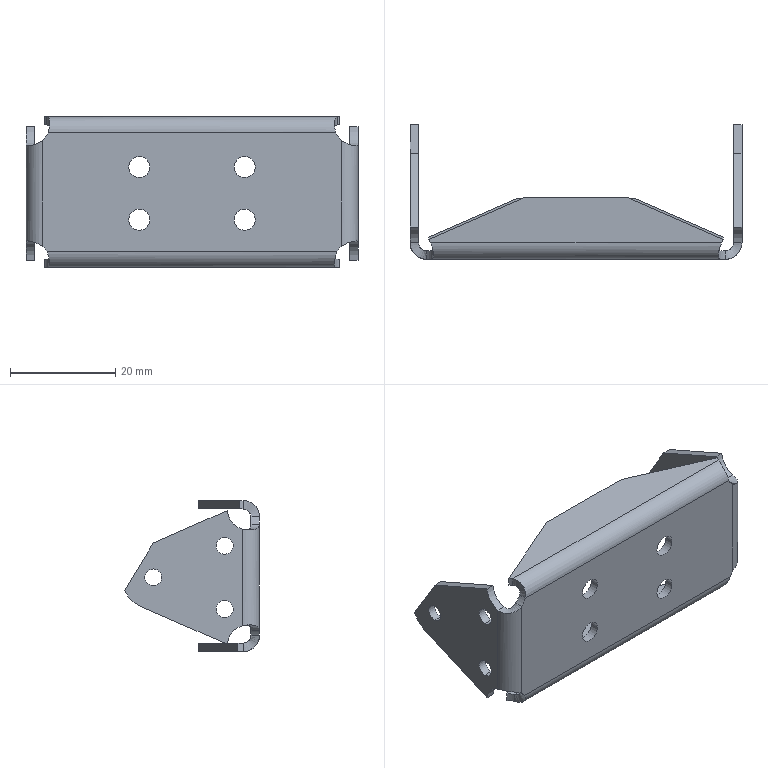Part | SolidWorks | features BaseBody 1 | 1 solid | 72 faces | box 63 x 25.588 x 28.631 mm | volume 5001 mm3 | cylinder 42 | plane 22 | spline 8 | commonest cylinder face diameters 3.2 x14 8 x12 4 x8 6.4 x2 12 x2 2.8 x1